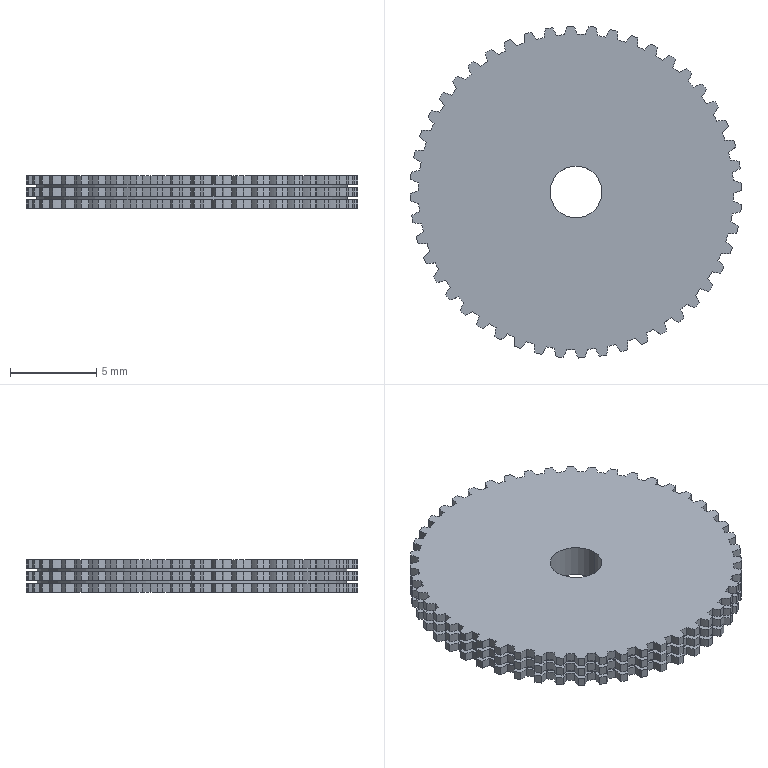Part | SolidWorks | features ICE 7, CirPattern 3, Cut 1, Extrusion 1 | 1 solid | 594 faces | box 19.259 x 19.259 x 1.9 mm | volume 502.853 mm3 | cylinder 588 | plane 6 | commonest cylinder face diameters 6.396 x294 18.3 x144 19.26 x144 18 x4 3 x2